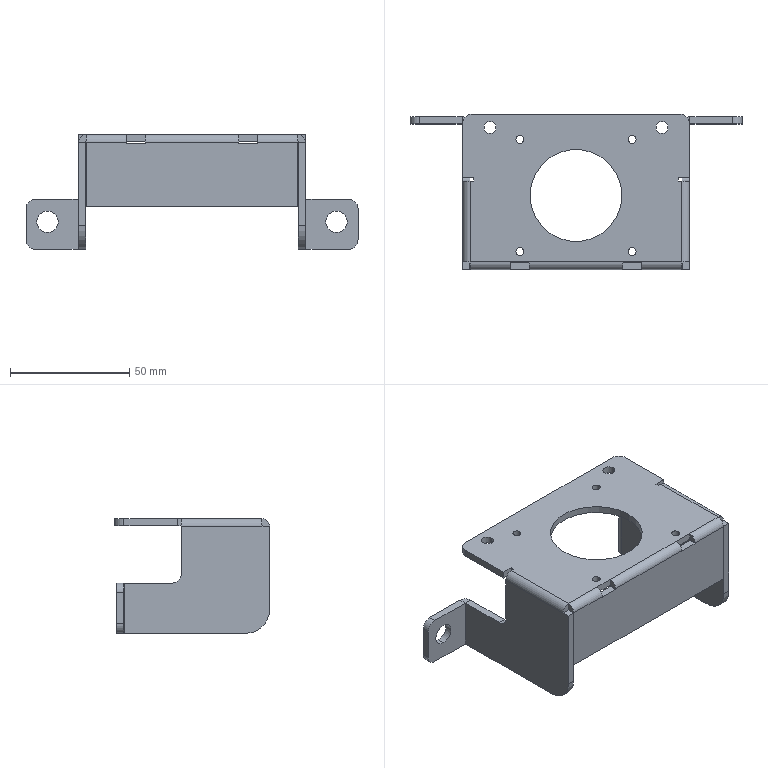Part | STEP file | 1 solid | 102 faces | box 139 x 65 x 48 mm | volume 36917 mm3 | plane 60 | cylinder 42 | commonest cylinder face diameters 3.3 x8 8 x8 0.4 x7 6.4 x7 5 x4 9 x4